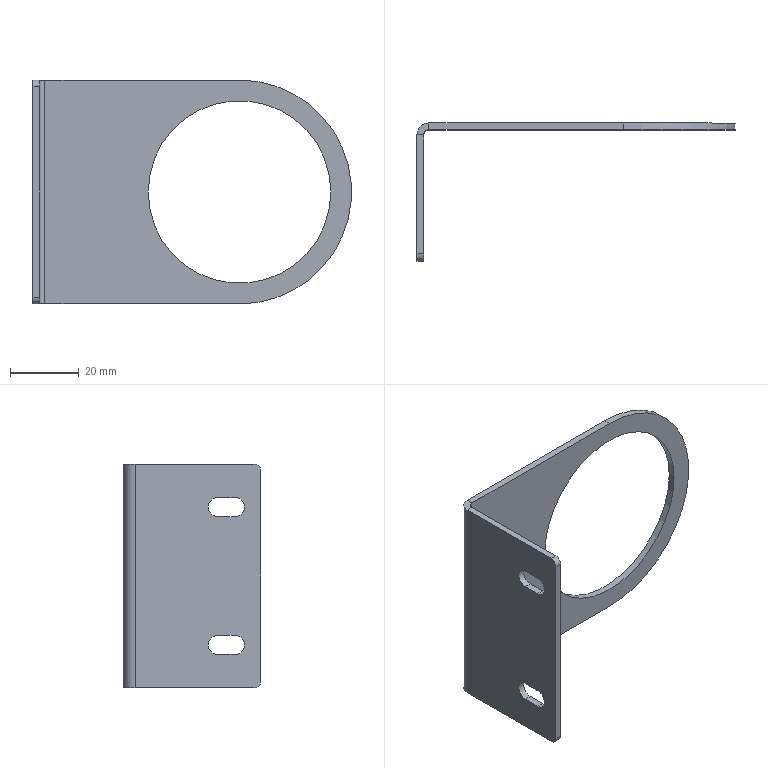Part | SolidWorks | features ICE 2, Fillet 1, FlatPattern 1, HoleWzd 1, SMBaseFlange 1, SheetMetal 1 | 1 solid | 26 faces | box 92.5 x 40 x 65 mm | volume 11298 mm3 | plane 15 | cylinder 11 | commonest cylinder face diameters 5.5 x4 4 x2 53 x2 3 x1 7 x1 65 x1
STEP:
#1=CARTESIAN_POINT('',(86.5,0.,0.));
#2=VERTEX_POINT('',#1);
#3=CARTESIAN_POINT('',(33.5,0.,0.));
#4=VERTEX_POINT('',#3);
#5=CARTESIAN_POINT('',(60.,0.,0.));
#6=DIRECTION('',(0.,1.,0.));
#7=DIRECTION('',(1.,0.,0.));
#8=AXIS2_PLACEMENT_3D('',#5,#6,#7);
#9=CIRCLE('',#8,26.5);
#10=EDGE_CURVE('',#2,#4,#9,.T.);
#11=ORIENTED_EDGE('',*,*,#10,.T.);
#12=CARTESIAN_POINT('',(33.5,-2.,0.));
#13=VERTEX_POINT('',#12);
#14=CARTESIAN_POINT('',(33.5,74.953,0.));
#15=DIRECTION('',(0.,-1.,0.));
#16=VECTOR('',#15,1000.);
#17=LINE('',#14,#16);
#18=EDGE_CURVE('',#4,#13,#17,.T.);
#19=ORIENTED_EDGE('',*,*,#18,.T.);
#20=CARTESIAN_POINT('',(86.5,-2.,0.));
#21=VERTEX_POINT('',#20);
#22=CARTESIAN_POINT('',(60.,-2.,0.));
#23=DIRECTION('',(0.,-1.,0.));
#24=DIRECTION('',(1.,0.,0.));
#25=AXIS2_PLACEMENT_3D('',#22,#23,#24);
#26=CIRCLE('',#25,26.5);
#27=EDGE_CURVE('',#13,#21,#26,.T.);
#28=ORIENTED_EDGE('',*,*,#27,.T.);
#29=CARTESIAN_POINT('',(86.5,74.953,0.));
#30=DIRECTION('',(0.,-1.,0.));
#31=VECTOR('',#30,1000.);
#32=LINE('',#29,#31);
#33=EDGE_CURVE('',#2,#21,#32,.T.);
#34=ORIENTED_EDGE('',*,*,#33,.F.);
#35=EDGE_LOOP('',(#11,#19,#28,#34));
#36=FACE_OUTER_BOUND('',#35,.T.);
#37=CARTESIAN_POINT('',(60.,74.953,0.));
#38=DIRECTION('',(0.,-1.,0.));
#39=DIRECTION('',(1.,0.,0.));
#40=AXIS2_PLACEMENT_3D('',#37,#38,#39);
#41=CYLINDRICAL_SURFACE('',#40,26.5);
#42=ADVANCED_FACE('',(#36),#41,.F.);
#43=CARTESIAN_POINT('',(3.5,0.,32.5));
#44=VERTEX_POINT('',#43);
#45=CARTESIAN_POINT('',(3.5,-2.,32.5));
#46=VERTEX_POINT('',#45);
#47=CARTESIAN_POINT('',(3.5,0.,32.5));
#48=DIRECTION('',(0.,-1.,0.));
#49=VECTOR('',#48,1000.);
#50=LINE('',#47,#49);
#51=EDGE_CURVE('',#44,#46,#50,.T.);
#52=ORIENTED_EDGE('',*,*,#51,.F.);
#53=CARTESIAN_POINT('',(0.,-3.5,32.5));
#54=VERTEX_POINT('',#53);
#55=CARTESIAN_POINT('',(3.5,-3.5,32.5));
#56=DIRECTION('',(0.,0.,1.));
#57=DIRECTION('',(-1.,0.,0.));
#58=AXIS2_PLACEMENT_3D('',#55,#56,#57);
#59=CIRCLE('',#58,3.5);
#60=EDGE_CURVE('',#44,#54,#59,.T.);
#61=ORIENTED_EDGE('',*,*,#60,.T.);
#62=CARTESIAN_POINT('',(2.,-3.5,32.5));
#63=VERTEX_POINT('',#62);
#64=CARTESIAN_POINT('',(2.,-3.5,32.5));
#65=DIRECTION('',(-1.,0.,0.));
#66=VECTOR('',#65,1000.);
#67=LINE('',#64,#66);
#68=EDGE_CURVE('',#63,#54,#67,.T.);
#69=ORIENTED_EDGE('',*,*,#68,.F.);
#70=CARTESIAN_POINT('',(3.5,-3.5,32.5));
#71=DIRECTION('',(0.,0.,1.));
#72=DIRECTION('',(1.,0.,0.));
#73=AXIS2_PLACEMENT_3D('',#70,#71,#72);
#74=CIRCLE('',#73,1.5);
#75=EDGE_CURVE('',#46,#63,#74,.T.);
#76=ORIENTED_EDGE('',*,*,#75,.F.);
#77=EDGE_LOOP('',(#52,#61,#69,#76));
#78=FACE_OUTER_BOUND('',#77,.T.);
#79=CARTESIAN_POINT('',(3.5,0.,32.5));
#80=DIRECTION('',(0.,0.,1.));
#81=DIRECTION('',(1.,0.,0.));
#82=AXIS2_PLACEMENT_3D('',#79,#80,#81);
#83=PLANE('',#82);
#84=ADVANCED_FACE('',(#78),#83,.T.);
#85=CARTESIAN_POINT('',(60.,0.,32.5));
#86=VERTEX_POINT('',#85);
#87=CARTESIAN_POINT('',(60.,0.,32.5));
#88=DIRECTION('',(-1.,0.,0.));
#89=VECTOR('',#88,1000.);
#90=LINE('',#87,#89);
#91=EDGE_CURVE('',#86,#44,#90,.T.);
#92=ORIENTED_EDGE('',*,*,#91,.T.);
#93=ORIENTED_EDGE('',*,*,#51,.T.);
#94=CARTESIAN_POINT('',(60.,-2.,32.5));
#95=VERTEX_POINT('',#94);
#96=CARTESIAN_POINT('',(60.,-2.,32.5));
#97=DIRECTION('',(-1.,0.,0.));
#98=VECTOR('',#97,1000.);
#99=LINE('',#96,#98);
#100=EDGE_CURVE('',#95,#46,#99,.T.);
#101=ORIENTED_EDGE('',*,*,#100,.F.);
#102=CARTESIAN_POINT('',(60.,0.,32.5));
#103=DIRECTION('',(0.,-1.,0.));
#104=VECTOR('',#103,1000.);
#105=LINE('',#102,#104);
#106=EDGE_CURVE('',#86,#95,#105,.T.);
#107=ORIENTED_EDGE('',*,*,#106,.F.);
#108=EDGE_LOOP('',(#92,#93,#101,#107));
#109=FACE_OUTER_BOUND('',#108,.T.);
#110=CARTESIAN_POINT('',(2.,-3.5,32.5));
#111=DIRECTION('',(0.,0.,1.));
#112=DIRECTION('',(1.,0.,0.));
#113=AXIS2_PLACEMENT_3D('',#110,#111,#112);
#114=PLANE('',#113);
#115=ADVANCED_FACE('',(#109),#114,.T.);
#116=CARTESIAN_POINT('',(0.,-3.5,-32.5));
#117=VERTEX_POINT('',#116);
#118=CARTESIAN_POINT('',(2.,-3.5,-32.5));
#119=VERTEX_POINT('',#118);
#120=CARTESIAN_POINT('',(0.,-3.5,-32.5));
#121=DIRECTION('',(1.,0.,0.));
#122=VECTOR('',#121,1000.);
#123=LINE('',#120,#122);
#124=EDGE_CURVE('',#117,#119,#123,.T.);
#125=ORIENTED_EDGE('',*,*,#124,.F.);
#126=CARTESIAN_POINT('',(3.5,0.,-32.5));
#127=VERTEX_POINT('',#126);
#128=CARTESIAN_POINT('',(3.5,-3.5,-32.5));
#129=DIRECTION('',(0.,0.,1.));
#130=DIRECTION('',(-1.,0.,0.));
#131=AXIS2_PLACEMENT_3D('',#128,#129,#130);
#132=CIRCLE('',#131,3.5);
#133=EDGE_CURVE('',#127,#117,#132,.T.);
#134=ORIENTED_EDGE('',*,*,#133,.F.);
#135=CARTESIAN_POINT('',(3.5,-2.,-32.5));
#136=VERTEX_POINT('',#135);
#137=CARTESIAN_POINT('',(3.5,-2.,-32.5));
#138=DIRECTION('',(0.,1.,0.));
#139=VECTOR('',#138,1000.);
#140=LINE('',#137,#139);
#141=EDGE_CURVE('',#136,#127,#140,.T.);
#142=ORIENTED_EDGE('',*,*,#141,.F.);
#143=CARTESIAN_POINT('',(3.5,-3.5,-32.5));
#144=DIRECTION('',(0.,0.,1.));
#145=DIRECTION('',(1.,0.,0.));
#146=AXIS2_PLACEMENT_3D('',#143,#144,#145);
#147=CIRCLE('',#146,1.5);
#148=EDGE_CURVE('',#136,#119,#147,.T.);
#149=ORIENTED_EDGE('',*,*,#148,.T.);
#150=EDGE_LOOP('',(#125,#134,#142,#149));
#151=FACE_OUTER_BOUND('',#150,.T.);
#152=CARTESIAN_POINT('',(0.,-3.5,-32.5));
#153=DIRECTION('',(0.,0.,-1.));
#154=DIRECTION('',(-1.,0.,0.));
#155=AXIS2_PLACEMENT_3D('',#152,#153,#154);
#156=PLANE('',#155);
#157=ADVANCED_FACE('',(#151),#156,.T.);
#158=CARTESIAN_POINT('',(2.,-38.,-32.5));
#159=VERTEX_POINT('',#158);
#160=CARTESIAN_POINT('',(2.,0.,-32.5));
#161=DIRECTION('',(0.,-1.,0.));
#162=VECTOR('',#161,1000.);
#163=LINE('',#160,#162);
#164=EDGE_CURVE('',#119,#159,#163,.T.);
#165=ORIENTED_EDGE('',*,*,#164,.T.);
#166=CARTESIAN_POINT('',(0.,-38.,-32.5));
#167=VERTEX_POINT('',#166);
#168=CARTESIAN_POINT('',(3.5,-38.,-32.5));
#169=DIRECTION('',(-1.,0.,0.));
#170=VECTOR('',#169,1000.);
#171=LINE('',#168,#170);
#172=EDGE_CURVE('',#159,#167,#171,.T.);
#173=ORIENTED_EDGE('',*,*,#172,.T.);
#174=CARTESIAN_POINT('',(0.,0.,-32.5));
#175=DIRECTION('',(0.,-1.,0.));
#176=VECTOR('',#175,1000.);
#177=LINE('',#174,#176);
#178=EDGE_CURVE('',#117,#167,#177,.T.);
#179=ORIENTED_EDGE('',*,*,#178,.F.);
#180=ORIENTED_EDGE('',*,*,#124,.T.);
#181=EDGE_LOOP('',(#165,#173,#179,#180));
#182=FACE_OUTER_BOUND('',#181,.T.);
#183=CARTESIAN_POINT('',(3.5,-2.,-32.5));
#184=DIRECTION('',(0.,0.,-1.));
#185=DIRECTION('',(-1.,0.,0.));
#186=AXIS2_PLACEMENT_3D('',#183,#184,#185);
#187=PLANE('',#186);
#188=ADVANCED_FACE('',(#182),#187,.T.);
#189=CARTESIAN_POINT('',(0.,-32.5,22.75));
#190=VERTEX_POINT('',#189);
#191=CARTESIAN_POINT('',(0.,-27.5,22.75));
#192=VERTEX_POINT('',#191);
#193=CARTESIAN_POINT('',(0.,-32.5,22.75));
#194=DIRECTION('',(0.,1.,0.));
#195=VECTOR('',#194,1000.);
#196=LINE('',#193,#195);
#197=EDGE_CURVE('',#190,#192,#196,.T.);
#198=ORIENTED_EDGE('',*,*,#197,.F.);
#199=CARTESIAN_POINT('',(0.,-32.5,17.25));
#200=VERTEX_POINT('',#199);
#201=CARTESIAN_POINT('',(0.,-32.5,20.));
#202=DIRECTION('',(1.,0.,0.));
#203=DIRECTION('',(0.,0.,-1.));
#204=AXIS2_PLACEMENT_3D('',#201,#202,#203);
#205=CIRCLE('',#204,2.75);
#206=EDGE_CURVE('',#190,#200,#205,.T.);
#207=ORIENTED_EDGE('',*,*,#206,.T.);
#208=CARTESIAN_POINT('',(0.,-27.5,17.25));
#209=VERTEX_POINT('',#208);
#210=CARTESIAN_POINT('',(0.,-32.5,17.25));
#211=DIRECTION('',(0.,1.,0.));
#212=VECTOR('',#211,1000.);
#213=LINE('',#210,#212);
#214=EDGE_CURVE('',#200,#209,#213,.T.);
#215=ORIENTED_EDGE('',*,*,#214,.T.);
#216=CARTESIAN_POINT('',(0.,-27.5,20.));
#217=DIRECTION('',(1.,0.,0.));
#218=DIRECTION('',(0.,0.,-1.));
#219=AXIS2_PLACEMENT_3D('',#216,#217,#218);
#220=CIRCLE('',#219,2.75);
#221=EDGE_CURVE('',#209,#192,#220,.T.);
#222=ORIENTED_EDGE('',*,*,#221,.T.);
#223=EDGE_LOOP('',(#198,#207,#215,#222));
#224=FACE_BOUND('',#223,.T.);
#225=CARTESIAN_POINT('',(0.,-32.5,-17.25));
#226=VERTEX_POINT('',#225);
#227=CARTESIAN_POINT('',(0.,-32.5,-22.75));
#228=VERTEX_POINT('',#227);
#229=CARTESIAN_POINT('',(0.,-32.5,-20.));
#230=DIRECTION('',(1.,0.,0.));
#231=DIRECTION('',(0.,0.,-1.));
#232=AXIS2_PLACEMENT_3D('',#229,#230,#231);
#233=CIRCLE('',#232,2.75);
#234=EDGE_CURVE('',#226,#228,#233,.T.);
#235=ORIENTED_EDGE('',*,*,#234,.T.);
#236=CARTESIAN_POINT('',(0.,-27.5,-22.75));
#237=VERTEX_POINT('',#236);
#238=CARTESIAN_POINT('',(0.,-32.5,-22.75));
#239=DIRECTION('',(0.,1.,0.));
#240=VECTOR('',#239,1000.);
#241=LINE('',#238,#240);
#242=EDGE_CURVE('',#228,#237,#241,.T.);
#243=ORIENTED_EDGE('',*,*,#242,.T.);
#244=CARTESIAN_POINT('',(0.,-27.5,-17.25));
#245=VERTEX_POINT('',#244);
#246=CARTESIAN_POINT('',(0.,-27.5,-20.));
#247=DIRECTION('',(1.,0.,0.));
#248=DIRECTION('',(0.,0.,-1.));
#249=AXIS2_PLACEMENT_3D('',#246,#247,#248);
#250=CIRCLE('',#249,2.75);
#251=EDGE_CURVE('',#237,#245,#250,.T.);
#252=ORIENTED_EDGE('',*,*,#251,.T.);
#253=CARTESIAN_POINT('',(0.,-32.5,-17.25));
#254=DIRECTION('',(0.,1.,0.));
#255=VECTOR('',#254,1000.);
#256=LINE('',#253,#255);
#257=EDGE_CURVE('',#226,#245,#256,.T.);
#258=ORIENTED_EDGE('',*,*,#257,.F.);
#259=EDGE_LOOP('',(#235,#243,#252,#258));
#260=FACE_BOUND('',#259,.T.);
#261=ORIENTED_EDGE('',*,*,#178,.T.);
#262=CARTESIAN_POINT('',(0.,-40.,-30.5));
#263=VERTEX_POINT('',#262);
#264=CARTESIAN_POINT('',(0.,-38.,-30.5));
#265=DIRECTION('',(-1.,0.,0.));
#266=DIRECTION('',(0.,1.,0.));
#267=AXIS2_PLACEMENT_3D('',#264,#265,#266);
#268=CIRCLE('',#267,2.);
#269=EDGE_CURVE('',#167,#263,#268,.T.);
#270=ORIENTED_EDGE('',*,*,#269,.T.);
#271=CARTESIAN_POINT('',(0.,-40.,30.5));
#272=VERTEX_POINT('',#271);
#273=CARTESIAN_POINT('',(0.,-40.,32.5));
#274=DIRECTION('',(0.,0.,-1.));
#275=VECTOR('',#274,1000.);
#276=LINE('',#273,#275);
#277=EDGE_CURVE('',#272,#263,#276,.T.);
#278=ORIENTED_EDGE('',*,*,#277,.F.);
#279=CARTESIAN_POINT('',(0.,-38.,32.5));
#280=VERTEX_POINT('',#279);
#281=CARTESIAN_POINT('',(0.,-38.,30.5));
#282=DIRECTION('',(-1.,0.,0.));
#283=DIRECTION('',(0.,1.,0.));
#284=AXIS2_PLACEMENT_3D('',#281,#282,#283);
#285=CIRCLE('',#284,2.);
#286=EDGE_CURVE('',#272,#280,#285,.T.);
#287=ORIENTED_EDGE('',*,*,#286,.T.);
#288=CARTESIAN_POINT('',(0.,0.,32.5));
#289=DIRECTION('',(0.,-1.,0.));
#290=VECTOR('',#289,1000.);
#291=LINE('',#288,#290);
#292=EDGE_CURVE('',#54,#280,#291,.T.);
#293=ORIENTED_EDGE('',*,*,#292,.F.);
#294=CARTESIAN_POINT('',(0.,-3.5,32.5));
#295=DIRECTION('',(0.,0.,-1.));
#296=VECTOR('',#295,1000.);
#297=LINE('',#294,#296);
#298=EDGE_CURVE('',#54,#117,#297,.T.);
#299=ORIENTED_EDGE('',*,*,#298,.T.);
#300=EDGE_LOOP('',(#261,#270,#278,#287,#293,#299));
#301=FACE_OUTER_BOUND('',#300,.T.);
#302=CARTESIAN_POINT('',(0.,0.,32.5));
#303=DIRECTION('',(1.,0.,0.));
#304=DIRECTION('',(0.,1.,0.));
#305=AXIS2_PLACEMENT_3D('',#302,#303,#304);
#306=PLANE('',#305);
#307=ADVANCED_FACE('',(#224,#260,#301),#306,.F.);
#308=ORIENTED_EDGE('',*,*,#277,.T.);
#309=CARTESIAN_POINT('',(2.,-40.,-30.5));
#310=VERTEX_POINT('',#309);
#311=CARTESIAN_POINT('',(2.,-40.,-30.5));
#312=DIRECTION('',(1.,0.,0.));
#313=VECTOR('',#312,1000.);
#314=LINE('',#311,#313);
#315=EDGE_CURVE('',#263,#310,#314,.T.);
#316=ORIENTED_EDGE('',*,*,#315,.T.);
#317=CARTESIAN_POINT('',(2.,-40.,30.5));
#318=VERTEX_POINT('',#317);
#319=CARTESIAN_POINT('',(2.,-40.,32.5));
#320=DIRECTION('',(0.,0.,-1.));
#321=VECTOR('',#320,1000.);
#322=LINE('',#319,#321);
#323=EDGE_CURVE('',#318,#310,#322,.T.);
#324=ORIENTED_EDGE('',*,*,#323,.F.);
#325=CARTESIAN_POINT('',(2.,-40.,30.5));
#326=DIRECTION('',(-1.,0.,0.));
#327=VECTOR('',#326,1000.);
#328=LINE('',#325,#327);
#329=EDGE_CURVE('',#318,#272,#328,.T.);
#330=ORIENTED_EDGE('',*,*,#329,.T.);
#331=EDGE_LOOP('',(#308,#316,#324,#330));
#332=FACE_OUTER_BOUND('',#331,.T.);
#333=CARTESIAN_POINT('',(2.,-40.,32.5));
#334=DIRECTION('',(0.,-1.,0.));
#335=DIRECTION('',(0.,0.,-1.));
#336=AXIS2_PLACEMENT_3D('',#333,#334,#335);
#337=PLANE('',#336);
#338=ADVANCED_FACE('',(#332),#337,.T.);
#339=CARTESIAN_POINT('',(2.,-32.5,22.75));
#340=VERTEX_POINT('',#339);
#341=CARTESIAN_POINT('',(2.,-32.5,17.25));
#342=VERTEX_POINT('',#341);
#343=CARTESIAN_POINT('',(2.,-32.5,20.));
#344=DIRECTION('',(1.,0.,0.));
#345=DIRECTION('',(0.,0.,-1.));
#346=AXIS2_PLACEMENT_3D('',#343,#344,#345);
#347=CIRCLE('',#346,2.75);
#348=EDGE_CURVE('',#340,#342,#347,.T.);
#349=ORIENTED_EDGE('',*,*,#348,.F.);
#350=CARTESIAN_POINT('',(2.,-27.5,22.75));
#351=VERTEX_POINT('',#350);
#352=CARTESIAN_POINT('',(2.,-32.5,22.75));
#353=DIRECTION('',(0.,1.,0.));
#354=VECTOR('',#353,1000.);
#355=LINE('',#352,#354);
#356=EDGE_CURVE('',#340,#351,#355,.T.);
#357=ORIENTED_EDGE('',*,*,#356,.T.);
#358=CARTESIAN_POINT('',(2.,-27.5,17.25));
#359=VERTEX_POINT('',#358);
#360=CARTESIAN_POINT('',(2.,-27.5,20.));
#361=DIRECTION('',(1.,0.,0.));
#362=DIRECTION('',(0.,0.,-1.));
#363=AXIS2_PLACEMENT_3D('',#360,#361,#362);
#364=CIRCLE('',#363,2.75);
#365=EDGE_CURVE('',#359,#351,#364,.T.);
#366=ORIENTED_EDGE('',*,*,#365,.F.);
#367=CARTESIAN_POINT('',(2.,-32.5,17.25));
#368=DIRECTION('',(0.,1.,0.));
#369=VECTOR('',#368,1000.);
#370=LINE('',#367,#369);
#371=EDGE_CURVE('',#342,#359,#370,.T.);
#372=ORIENTED_EDGE('',*,*,#371,.F.);
#373=EDGE_LOOP('',(#349,#357,#366,#372));
#374=FACE_BOUND('',#373,.T.);
#375=CARTESIAN_POINT('',(2.,-27.5,-22.75));
#376=VERTEX_POINT('',#375);
#377=CARTESIAN_POINT('',(2.,-27.5,-17.25));
#378=VERTEX_POINT('',#377);
#379=CARTESIAN_POINT('',(2.,-27.5,-20.));
#380=DIRECTION('',(1.,0.,0.));
#381=DIRECTION('',(0.,0.,-1.));
#382=AXIS2_PLACEMENT_3D('',#379,#380,#381);
#383=CIRCLE('',#382,2.75);
#384=EDGE_CURVE('',#376,#378,#383,.T.);
#385=ORIENTED_EDGE('',*,*,#384,.F.);
#386=CARTESIAN_POINT('',(2.,-32.5,-22.75));
#387=VERTEX_POINT('',#386);
#388=CARTESIAN_POINT('',(2.,-32.5,-22.75));
#389=DIRECTION('',(0.,1.,0.));
#390=VECTOR('',#389,1000.);
#391=LINE('',#388,#390);
#392=EDGE_CURVE('',#387,#376,#391,.T.);
#393=ORIENTED_EDGE('',*,*,#392,.F.);
#394=CARTESIAN_POINT('',(2.,-32.5,-17.25));
#395=VERTEX_POINT('',#394);
#396=CARTESIAN_POINT('',(2.,-32.5,-20.));
#397=DIRECTION('',(1.,0.,0.));
#398=DIRECTION('',(0.,0.,-1.));
#399=AXIS2_PLACEMENT_3D('',#396,#397,#398);
#400=CIRCLE('',#399,2.75);
#401=EDGE_CURVE('',#395,#387,#400,.T.);
#402=ORIENTED_EDGE('',*,*,#401,.F.);
#403=CARTESIAN_POINT('',(2.,-32.5,-17.25));
#404=DIRECTION('',(0.,1.,0.));
#405=VECTOR('',#404,1000.);
#406=LINE('',#403,#405);
#407=EDGE_CURVE('',#395,#378,#406,.T.);
#408=ORIENTED_EDGE('',*,*,#407,.T.);
#409=EDGE_LOOP('',(#385,#393,#402,#408));
#410=FACE_BOUND('',#409,.T.);
#411=ORIENTED_EDGE('',*,*,#323,.T.);
#412=CARTESIAN_POINT('',(2.,-38.,-30.5));
#413=DIRECTION('',(1.,0.,0.));
#414=DIRECTION('',(0.,1.,0.));
#415=AXIS2_PLACEMENT_3D('',#412,#413,#414);
#416=CIRCLE('',#415,2.);
#417=EDGE_CURVE('',#310,#159,#416,.T.);
#418=ORIENTED_EDGE('',*,*,#417,.T.);
#419=ORIENTED_EDGE('',*,*,#164,.F.);
#420=CARTESIAN_POINT('',(2.,-3.5,32.5));
#421=DIRECTION('',(0.,0.,-1.));
#422=VECTOR('',#421,1000.);
#423=LINE('',#420,#422);
#424=EDGE_CURVE('',#63,#119,#423,.T.);
#425=ORIENTED_EDGE('',*,*,#424,.F.);
#426=CARTESIAN_POINT('',(2.,-38.,32.5));
#427=VERTEX_POINT('',#426);
#428=CARTESIAN_POINT('',(2.,0.,32.5));
#429=DIRECTION('',(0.,-1.,0.));
#430=VECTOR('',#429,1000.);
#431=LINE('',#428,#430);
#432=EDGE_CURVE('',#63,#427,#431,.T.);
#433=ORIENTED_EDGE('',*,*,#432,.T.);
#434=CARTESIAN_POINT('',(2.,-38.,30.5));
#435=DIRECTION('',(1.,0.,0.));
#436=DIRECTION('',(0.,1.,0.));
#437=AXIS2_PLACEMENT_3D('',#434,#435,#436);
#438=CIRCLE('',#437,2.);
#439=EDGE_CURVE('',#427,#318,#438,.T.);
#440=ORIENTED_EDGE('',*,*,#439,.T.);
#441=EDGE_LOOP('',(#411,#418,#419,#425,#433,#440));
#442=FACE_OUTER_BOUND('',#441,.T.);
#443=CARTESIAN_POINT('',(2.,0.,32.5));
#444=DIRECTION('',(1.,0.,0.));
#445=DIRECTION('',(0.,1.,0.));
#446=AXIS2_PLACEMENT_3D('',#443,#444,#445);
#447=PLANE('',#446);
#448=ADVANCED_FACE('',(#374,#410,#442),#447,.T.);
#449=ORIENTED_EDGE('',*,*,#148,.F.);
#450=CARTESIAN_POINT('',(3.5,-2.,32.5));
#451=DIRECTION('',(0.,0.,-1.));
#452=VECTOR('',#451,1000.);
#453=LINE('',#450,#452);
#454=EDGE_CURVE('',#46,#136,#453,.T.);
#455=ORIENTED_EDGE('',*,*,#454,.F.);
#456=ORIENTED_EDGE('',*,*,#75,.T.);
#457=ORIENTED_EDGE('',*,*,#424,.T.);
#458=EDGE_LOOP('',(#449,#455,#456,#457));
#459=FACE_OUTER_BOUND('',#458,.T.);
#460=CARTESIAN_POINT('',(3.5,-3.5,32.5));
#461=DIRECTION('',(0.,0.,-1.));
#462=DIRECTION('',(-1.,0.,0.));
#463=AXIS2_PLACEMENT_3D('',#460,#461,#462);
#464=CYLINDRICAL_SURFACE('',#463,1.5);
#465=ADVANCED_FACE('',(#459),#464,.F.);
#466=CARTESIAN_POINT('',(60.,-2.,0.));
#467=DIRECTION('',(0.,-1.,0.));
#468=DIRECTION('',(1.,0.,0.));
#469=AXIS2_PLACEMENT_3D('',#466,#467,#468);
#470=CIRCLE('',#469,26.5);
#471=EDGE_CURVE('',#21,#13,#470,.T.);
#472=ORIENTED_EDGE('',*,*,#471,.F.);
#473=ORIENTED_EDGE('',*,*,#27,.F.);
#474=EDGE_LOOP('',(#472,#473));
#475=FACE_BOUND('',#474,.T.);
#476=CARTESIAN_POINT('',(60.,-2.,-32.5));
#477=VERTEX_POINT('',#476);
#478=CARTESIAN_POINT('',(60.,-2.,-32.5));
#479=DIRECTION('',(-1.,0.,0.));
#480=VECTOR('',#479,1000.);
#481=LINE('',#478,#480);
#482=EDGE_CURVE('',#477,#136,#481,.T.);
#483=ORIENTED_EDGE('',*,*,#482,.F.);
#484=CARTESIAN_POINT('',(60.,-2.,0.));
#485=DIRECTION('',(0.,1.,0.));
#486=DIRECTION('',(1.,0.,0.));
#487=AXIS2_PLACEMENT_3D('',#484,#485,#486);
#488=CIRCLE('',#487,32.5);
#489=EDGE_CURVE('',#95,#477,#488,.T.);
#490=ORIENTED_EDGE('',*,*,#489,.F.);
#491=ORIENTED_EDGE('',*,*,#100,.T.);
#492=ORIENTED_EDGE('',*,*,#454,.T.);
#493=EDGE_LOOP('',(#483,#490,#491,#492));
#494=FACE_OUTER_BOUND('',#493,.T.);
#495=CARTESIAN_POINT('',(60.,-2.,32.5));
#496=DIRECTION('',(0.,-1.,0.));
#497=DIRECTION('',(1.,0.,0.));
#498=AXIS2_PLACEMENT_3D('',#495,#496,#497);
#499=PLANE('',#498);
#500=ADVANCED_FACE('',(#475,#494),#499,.T.);
#501=ORIENTED_EDGE('',*,*,#10,.F.);
#502=CARTESIAN_POINT('',(60.,0.,0.));
#503=DIRECTION('',(0.,1.,0.));
#504=DIRECTION('',(1.,0.,0.));
#505=AXIS2_PLACEMENT_3D('',#502,#503,#504);
#506=CIRCLE('',#505,26.5);
#507=EDGE_CURVE('',#4,#2,#506,.T.);
#508=ORIENTED_EDGE('',*,*,#507,.F.);
#509=EDGE_LOOP('',(#501,#508));
#510=FACE_BOUND('',#509,.T.);
#511=ORIENTED_EDGE('',*,*,#91,.F.);
#512=CARTESIAN_POINT('',(60.,0.,-32.5));
#513=VERTEX_POINT('',#512);
#514=CARTESIAN_POINT('',(60.,0.,0.));
#515=DIRECTION('',(0.,1.,0.));
#516=DIRECTION('',(-1.,0.,0.));
#517=AXIS2_PLACEMENT_3D('',#514,#515,#516);
#518=CIRCLE('',#517,32.5);
#519=EDGE_CURVE('',#86,#513,#518,.T.);
#520=ORIENTED_EDGE('',*,*,#519,.T.);
#521=CARTESIAN_POINT('',(60.,0.,-32.5));
#522=DIRECTION('',(-1.,0.,0.));
#523=VECTOR('',#522,1000.);
#524=LINE('',#521,#523);
#525=EDGE_CURVE('',#513,#127,#524,.T.);
#526=ORIENTED_EDGE('',*,*,#525,.T.);
#527=CARTESIAN_POINT('',(3.5,0.,32.5));
#528=DIRECTION('',(0.,0.,-1.));
#529=VECTOR('',#528,1000.);
#530=LINE('',#527,#529);
#531=EDGE_CURVE('',#44,#127,#530,.T.);
#532=ORIENTED_EDGE('',*,*,#531,.F.);
#533=EDGE_LOOP('',(#511,#520,#526,#532));
#534=FACE_OUTER_BOUND('',#533,.T.);
#535=CARTESIAN_POINT('',(60.,0.,32.5));
#536=DIRECTION('',(0.,-1.,0.));
#537=DIRECTION('',(1.,0.,0.));
#538=AXIS2_PLACEMENT_3D('',#535,#536,#537);
#539=PLANE('',#538);
#540=ADVANCED_FACE('',(#510,#534),#539,.F.);
#541=ORIENTED_EDGE('',*,*,#133,.T.);
#542=ORIENTED_EDGE('',*,*,#298,.F.);
#543=ORIENTED_EDGE('',*,*,#60,.F.);
#544=ORIENTED_EDGE('',*,*,#531,.T.);
#545=EDGE_LOOP('',(#541,#542,#543,#544));
#546=FACE_OUTER_BOUND('',#545,.T.);
#547=CARTESIAN_POINT('',(3.5,-3.5,32.5));
#548=DIRECTION('',(0.,0.,-1.));
#549=DIRECTION('',(-1.,0.,0.));
#550=AXIS2_PLACEMENT_3D('',#547,#548,#549);
#551=CYLINDRICAL_SURFACE('',#550,3.5);
#552=ADVANCED_FACE('',(#546),#551,.T.);
#553=ORIENTED_EDGE('',*,*,#292,.T.);
#554=CARTESIAN_POINT('',(3.5,-38.,32.5));
#555=DIRECTION('',(1.,0.,0.));
#556=VECTOR('',#555,1000.);
#557=LINE('',#554,#556);
#558=EDGE_CURVE('',#280,#427,#557,.T.);
#559=ORIENTED_EDGE('',*,*,#558,.T.);
#560=ORIENTED_EDGE('',*,*,#432,.F.);
#561=ORIENTED_EDGE('',*,*,#68,.T.);
#562=EDGE_LOOP('',(#553,#559,#560,#561));
#563=FACE_OUTER_BOUND('',#562,.T.);
#564=CARTESIAN_POINT('',(3.5,-3.5,32.5));
#565=DIRECTION('',(0.,0.,1.));
#566=DIRECTION('',(1.,0.,0.));
#567=AXIS2_PLACEMENT_3D('',#564,#565,#566);
#568=PLANE('',#567);
#569=ADVANCED_FACE('',(#563),#568,.T.);
#570=ORIENTED_EDGE('',*,*,#482,.T.);
#571=ORIENTED_EDGE('',*,*,#141,.T.);
#572=ORIENTED_EDGE('',*,*,#525,.F.);
#573=CARTESIAN_POINT('',(60.,0.,-32.5));
#574=DIRECTION('',(0.,-1.,0.));
#575=VECTOR('',#574,1000.);
#576=LINE('',#573,#575);
#577=EDGE_CURVE('',#513,#477,#576,.T.);
#578=ORIENTED_EDGE('',*,*,#577,.T.);
#579=EDGE_LOOP('',(#570,#571,#572,#578));
#580=FACE_OUTER_BOUND('',#579,.T.);
#581=CARTESIAN_POINT('',(3.5,-3.5,-32.5));
#582=DIRECTION('',(0.,0.,1.));
#583=DIRECTION('',(1.,0.,0.));
#584=AXIS2_PLACEMENT_3D('',#581,#582,#583);
#585=PLANE('',#584);
#586=ADVANCED_FACE('',(#580),#585,.F.);
#587=ORIENTED_EDGE('',*,*,#519,.F.);
#588=ORIENTED_EDGE('',*,*,#106,.T.);
#589=ORIENTED_EDGE('',*,*,#489,.T.);
#590=ORIENTED_EDGE('',*,*,#577,.F.);
#591=EDGE_LOOP('',(#587,#588,#589,#590));
#592=FACE_OUTER_BOUND('',#591,.T.);
#593=CARTESIAN_POINT('',(60.,-93.924,0.));
#594=DIRECTION('',(0.,1.,0.));
#595=DIRECTION('',(-1.,0.,0.));
#596=AXIS2_PLACEMENT_3D('',#593,#594,#595);
#597=CYLINDRICAL_SURFACE('',#596,32.5);
#598=ADVANCED_FACE('',(#592),#597,.T.);
#599=ORIENTED_EDGE('',*,*,#18,.F.);
#600=ORIENTED_EDGE('',*,*,#507,.T.);
#601=ORIENTED_EDGE('',*,*,#33,.T.);
#602=ORIENTED_EDGE('',*,*,#471,.T.);
#603=EDGE_LOOP('',(#599,#600,#601,#602));
#604=FACE_OUTER_BOUND('',#603,.T.);
#605=CARTESIAN_POINT('',(60.,74.953,0.));
#606=DIRECTION('',(0.,-1.,0.));
#607=DIRECTION('',(1.,0.,0.));
#608=AXIS2_PLACEMENT_3D('',#605,#606,#607);
#609=CYLINDRICAL_SURFACE('',#608,26.5);
#610=ADVANCED_FACE('',(#604),#609,.F.);
#611=ORIENTED_EDGE('',*,*,#417,.F.);
#612=ORIENTED_EDGE('',*,*,#315,.F.);
#613=ORIENTED_EDGE('',*,*,#269,.F.);
#614=ORIENTED_EDGE('',*,*,#172,.F.);
#615=EDGE_LOOP('',(#611,#612,#613,#614));
#616=FACE_OUTER_BOUND('',#615,.T.);
#617=CARTESIAN_POINT('',(3.5,-38.,-30.5));
#618=DIRECTION('',(-1.,0.,0.));
#619=DIRECTION('',(0.,0.,1.));
#620=AXIS2_PLACEMENT_3D('',#617,#618,#619);
#621=CYLINDRICAL_SURFACE('',#620,2.);
#622=ADVANCED_FACE('',(#616),#621,.T.);
#623=ORIENTED_EDGE('',*,*,#439,.F.);
#624=ORIENTED_EDGE('',*,*,#558,.F.);
#625=ORIENTED_EDGE('',*,*,#286,.F.);
#626=ORIENTED_EDGE('',*,*,#329,.F.);
#627=EDGE_LOOP('',(#623,#624,#625,#626));
#628=FACE_OUTER_BOUND('',#627,.T.);
#629=CARTESIAN_POINT('',(2.,-38.,30.5));
#630=DIRECTION('',(-1.,0.,0.));
#631=DIRECTION('',(0.,0.,1.));
#632=AXIS2_PLACEMENT_3D('',#629,#630,#631);
#633=CYLINDRICAL_SURFACE('',#632,2.);
#634=ADVANCED_FACE('',(#628),#633,.T.);
#635=ORIENTED_EDGE('',*,*,#251,.F.);
#636=CARTESIAN_POINT('',(2.,-27.5,-22.75));
#637=DIRECTION('',(-1.,0.,0.));
#638=VECTOR('',#637,1000.);
#639=LINE('',#636,#638);
#640=EDGE_CURVE('',#376,#237,#639,.T.);
#641=ORIENTED_EDGE('',*,*,#640,.F.);
#642=ORIENTED_EDGE('',*,*,#384,.T.);
#643=CARTESIAN_POINT('',(2.,-27.5,-17.25));
#644=DIRECTION('',(1.,0.,0.));
#645=VECTOR('',#644,1000.);
#646=LINE('',#643,#645);
#647=EDGE_CURVE('',#245,#378,#646,.T.);
#648=ORIENTED_EDGE('',*,*,#647,.F.);
#649=EDGE_LOOP('',(#635,#641,#642,#648));
#650=FACE_OUTER_BOUND('',#649,.T.);
#651=CARTESIAN_POINT('',(2.,-27.5,-20.));
#652=DIRECTION('',(1.,0.,0.));
#653=DIRECTION('',(0.,0.,-1.));
#654=AXIS2_PLACEMENT_3D('',#651,#652,#653);
#655=CYLINDRICAL_SURFACE('',#654,2.75);
#656=ADVANCED_FACE('',(#650),#655,.F.);
#657=ORIENTED_EDGE('',*,*,#401,.T.);
#658=CARTESIAN_POINT('',(2.,-32.5,-22.75));
#659=DIRECTION('',(1.,0.,0.));
#660=VECTOR('',#659,1000.);
#661=LINE('',#658,#660);
#662=EDGE_CURVE('',#228,#387,#661,.T.);
#663=ORIENTED_EDGE('',*,*,#662,.F.);
#664=ORIENTED_EDGE('',*,*,#234,.F.);
#665=CARTESIAN_POINT('',(2.,-32.5,-17.25));
#666=DIRECTION('',(-1.,0.,0.));
#667=VECTOR('',#666,1000.);
#668=LINE('',#665,#667);
#669=EDGE_CURVE('',#395,#226,#668,.T.);
#670=ORIENTED_EDGE('',*,*,#669,.F.);
#671=EDGE_LOOP('',(#657,#663,#664,#670));
#672=FACE_OUTER_BOUND('',#671,.T.);
#673=CARTESIAN_POINT('',(2.,-32.5,-20.));
#674=DIRECTION('',(1.,0.,0.));
#675=DIRECTION('',(0.,0.,-1.));
#676=AXIS2_PLACEMENT_3D('',#673,#674,#675);
#677=CYLINDRICAL_SURFACE('',#676,2.75);
#678=ADVANCED_FACE('',(#672),#677,.F.);
#679=ORIENTED_EDGE('',*,*,#647,.T.);
#680=ORIENTED_EDGE('',*,*,#407,.F.);
#681=ORIENTED_EDGE('',*,*,#669,.T.);
#682=ORIENTED_EDGE('',*,*,#257,.T.);
#683=EDGE_LOOP('',(#679,#680,#681,#682));
#684=FACE_OUTER_BOUND('',#683,.T.);
#685=CARTESIAN_POINT('',(2.,-32.5,-17.25));
#686=DIRECTION('',(0.,0.,1.));
#687=DIRECTION('',(1.,0.,0.));
#688=AXIS2_PLACEMENT_3D('',#685,#686,#687);
#689=PLANE('',#688);
#690=ADVANCED_FACE('',(#684),#689,.F.);
#691=ORIENTED_EDGE('',*,*,#640,.T.);
#692=ORIENTED_EDGE('',*,*,#242,.F.);
#693=ORIENTED_EDGE('',*,*,#662,.T.);
#694=ORIENTED_EDGE('',*,*,#392,.T.);
#695=EDGE_LOOP('',(#691,#692,#693,#694));
#696=FACE_OUTER_BOUND('',#695,.T.);
#697=CARTESIAN_POINT('',(2.,-32.5,-22.75));
#698=DIRECTION('',(0.,0.,-1.));
#699=DIRECTION('',(-1.,0.,0.));
#700=AXIS2_PLACEMENT_3D('',#697,#698,#699);
#701=PLANE('',#700);
#702=ADVANCED_FACE('',(#696),#701,.F.);
#703=ORIENTED_EDGE('',*,*,#221,.F.);
#704=CARTESIAN_POINT('',(2.,-27.5,17.25));
#705=DIRECTION('',(-1.,0.,0.));
#706=VECTOR('',#705,1000.);
#707=LINE('',#704,#706);
#708=EDGE_CURVE('',#359,#209,#707,.T.);
#709=ORIENTED_EDGE('',*,*,#708,.F.);
#710=ORIENTED_EDGE('',*,*,#365,.T.);
#711=CARTESIAN_POINT('',(2.,-27.5,22.75));
#712=DIRECTION('',(1.,0.,0.));
#713=VECTOR('',#712,1000.);
#714=LINE('',#711,#713);
#715=EDGE_CURVE('',#192,#351,#714,.T.);
#716=ORIENTED_EDGE('',*,*,#715,.F.);
#717=EDGE_LOOP('',(#703,#709,#710,#716));
#718=FACE_OUTER_BOUND('',#717,.T.);
#719=CARTESIAN_POINT('',(2.,-27.5,20.));
#720=DIRECTION('',(1.,0.,0.));
#721=DIRECTION('',(0.,0.,-1.));
#722=AXIS2_PLACEMENT_3D('',#719,#720,#721);
#723=CYLINDRICAL_SURFACE('',#722,2.75);
#724=ADVANCED_FACE('',(#718),#723,.F.);
#725=ORIENTED_EDGE('',*,*,#348,.T.);
#726=CARTESIAN_POINT('',(2.,-32.5,17.25));
#727=DIRECTION('',(1.,0.,0.));
#728=VECTOR('',#727,1000.);
#729=LINE('',#726,#728);
#730=EDGE_CURVE('',#200,#342,#729,.T.);
#731=ORIENTED_EDGE('',*,*,#730,.F.);
#732=ORIENTED_EDGE('',*,*,#206,.F.);
#733=CARTESIAN_POINT('',(2.,-32.5,22.75));
#734=DIRECTION('',(-1.,0.,0.));
#735=VECTOR('',#734,1000.);
#736=LINE('',#733,#735);
#737=EDGE_CURVE('',#340,#190,#736,.T.);
#738=ORIENTED_EDGE('',*,*,#737,.F.);
#739=EDGE_LOOP('',(#725,#731,#732,#738));
#740=FACE_OUTER_BOUND('',#739,.T.);
#741=CARTESIAN_POINT('',(2.,-32.5,20.));
#742=DIRECTION('',(1.,0.,0.));
#743=DIRECTION('',(0.,0.,-1.));
#744=AXIS2_PLACEMENT_3D('',#741,#742,#743);
#745=CYLINDRICAL_SURFACE('',#744,2.75);
#746=ADVANCED_FACE('',(#740),#745,.F.);
#747=ORIENTED_EDGE('',*,*,#715,.T.);
#748=ORIENTED_EDGE('',*,*,#356,.F.);
#749=ORIENTED_EDGE('',*,*,#737,.T.);
#750=ORIENTED_EDGE('',*,*,#197,.T.);
#751=EDGE_LOOP('',(#747,#748,#749,#750));
#752=FACE_OUTER_BOUND('',#751,.T.);
#753=CARTESIAN_POINT('',(2.,-32.5,22.75));
#754=DIRECTION('',(0.,0.,1.));
#755=DIRECTION('',(1.,0.,0.));
#756=AXIS2_PLACEMENT_3D('',#753,#754,#755);
#757=PLANE('',#756);
#758=ADVANCED_FACE('',(#752),#757,.F.);
#759=ORIENTED_EDGE('',*,*,#708,.T.);
#760=ORIENTED_EDGE('',*,*,#214,.F.);
#761=ORIENTED_EDGE('',*,*,#730,.T.);
#762=ORIENTED_EDGE('',*,*,#371,.T.);
#763=EDGE_LOOP('',(#759,#760,#761,#762));
#764=FACE_OUTER_BOUND('',#763,.T.);
#765=CARTESIAN_POINT('',(2.,-32.5,17.25));
#766=DIRECTION('',(0.,0.,-1.));
#767=DIRECTION('',(-1.,0.,0.));
#768=AXIS2_PLACEMENT_3D('',#765,#766,#767);
#769=PLANE('',#768);
#770=ADVANCED_FACE('',(#764),#769,.F.);
#771=CLOSED_SHELL('',(#42,#84,#115,#157,#188,#307,#338,#448,#465,#500,#540,#552,#569,#586,#598,#610,#622,#634,#656,#678,#690,#702,#724,#746,#758,#770));
#772=MANIFOLD_SOLID_BREP('',#771);
#773=CARTESIAN_POINT('',(0.,0.,0.));
#774=DIRECTION('',(0.,0.,1.));
#775=DIRECTION('',(1.,0.,0.));
#776=AXIS2_PLACEMENT_3D('',#773,#774,#775);
#777=(LENGTH_UNIT()NAMED_UNIT(*)SI_UNIT(.MILLI.,.METRE.));
#778=UNCERTAINTY_MEASURE_WITH_UNIT(LENGTH_MEASURE(0.00001),#777,'','');
#779=(NAMED_UNIT(*)PLANE_ANGLE_UNIT()SI_UNIT($,.RADIAN.));
#780=(NAMED_UNIT(*)SI_UNIT($,.STERADIAN.)SOLID_ANGLE_UNIT());
#781=(GEOMETRIC_REPRESENTATION_CONTEXT(3)GLOBAL_UNCERTAINTY_ASSIGNED_CONTEXT((#778))GLOBAL_UNIT_ASSIGNED_CONTEXT((#777,#779,#780))REPRESENTATION_CONTEXT('',''));
#782=ADVANCED_BREP_SHAPE_REPRESENTATION('',(#772,#776),#781);